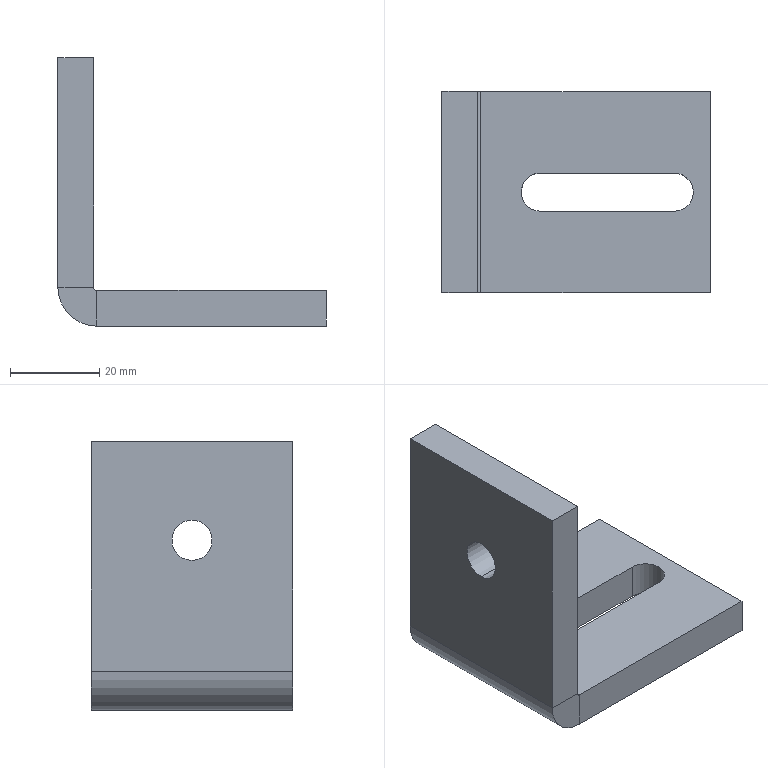Part | SolidWorks | features EdgeFlange 1, FlatPattern 1, HoleWzd 1, ICE 1, SMBaseFlange 1, SheetMetal 1 | 1 solid | 21 faces | box 60 x 45 x 60 mm | volume 36585 mm3 | plane 14 | cylinder 7 | commonest cylinder face diameters 8.5 x3 9 x2 1.473 x1 17.473 x1
STEP:
#1=CARTESIAN_POINT('',(64.788,13.156,0.));
#2=VERTEX_POINT('',#1);
#3=CARTESIAN_POINT('',(60.538,8.906,0.));
#4=VERTEX_POINT('',#3);
#5=CARTESIAN_POINT('',(64.788,8.906,0.));
#6=DIRECTION('',(0.,0.,1.));
#7=DIRECTION('',(1.,0.,0.));
#8=AXIS2_PLACEMENT_3D('',#5,#6,#7);
#9=CIRCLE('',#8,4.25);
#10=EDGE_CURVE('',#2,#4,#9,.T.);
#11=ORIENTED_EDGE('',*,*,#10,.T.);
#12=CARTESIAN_POINT('',(60.538,8.906,-8.));
#13=VERTEX_POINT('',#12);
#14=CARTESIAN_POINT('',(60.538,8.906,52.));
#15=DIRECTION('',(0.,0.,-1.));
#16=VECTOR('',#15,1000.);
#17=LINE('',#14,#16);
#18=EDGE_CURVE('',#4,#13,#17,.T.);
#19=ORIENTED_EDGE('',*,*,#18,.T.);
#20=CARTESIAN_POINT('',(64.788,13.156,-8.));
#21=VERTEX_POINT('',#20);
#22=CARTESIAN_POINT('',(64.788,8.906,-8.));
#23=DIRECTION('',(0.,0.,-1.));
#24=DIRECTION('',(-1.,0.,0.));
#25=AXIS2_PLACEMENT_3D('',#22,#23,#24);
#26=CIRCLE('',#25,4.25);
#27=EDGE_CURVE('',#13,#21,#26,.T.);
#28=ORIENTED_EDGE('',*,*,#27,.T.);
#29=CARTESIAN_POINT('',(64.788,13.156,52.));
#30=DIRECTION('',(0.,0.,-1.));
#31=VECTOR('',#30,1000.);
#32=LINE('',#29,#31);
#33=EDGE_CURVE('',#2,#21,#32,.T.);
#34=ORIENTED_EDGE('',*,*,#33,.F.);
#35=EDGE_LOOP('',(#11,#19,#28,#34));
#36=FACE_OUTER_BOUND('',#35,.T.);
#37=CARTESIAN_POINT('',(64.788,8.906,52.));
#38=DIRECTION('',(0.,0.,-1.));
#39=DIRECTION('',(-1.,0.,0.));
#40=AXIS2_PLACEMENT_3D('',#37,#38,#39);
#41=CYLINDRICAL_SURFACE('',#40,4.25);
#42=ADVANCED_FACE('',(#36),#41,.F.);
#43=CARTESIAN_POINT('',(42.788,8.906,34.5));
#44=VERTEX_POINT('',#43);
#45=CARTESIAN_POINT('',(42.788,8.906,25.5));
#46=VERTEX_POINT('',#45);
#47=CARTESIAN_POINT('',(42.788,8.906,30.));
#48=DIRECTION('',(1.,0.,0.));
#49=DIRECTION('',(0.,0.,-1.));
#50=AXIS2_PLACEMENT_3D('',#47,#48,#49);
#51=CIRCLE('',#50,4.5);
#52=EDGE_CURVE('',#44,#46,#51,.T.);
#53=ORIENTED_EDGE('',*,*,#52,.F.);
#54=CARTESIAN_POINT('',(50.788,8.906,34.5));
#55=VERTEX_POINT('',#54);
#56=CARTESIAN_POINT('',(50.788,8.906,34.5));
#57=DIRECTION('',(1.,0.,0.));
#58=VECTOR('',#57,1000.);
#59=LINE('',#56,#58);
#60=EDGE_CURVE('',#44,#55,#59,.T.);
#61=ORIENTED_EDGE('',*,*,#60,.T.);
#62=CARTESIAN_POINT('',(50.788,8.906,25.5));
#63=VERTEX_POINT('',#62);
#64=CARTESIAN_POINT('',(50.788,8.906,30.));
#65=DIRECTION('',(1.,0.,0.));
#66=DIRECTION('',(0.,0.,-1.));
#67=AXIS2_PLACEMENT_3D('',#64,#65,#66);
#68=CIRCLE('',#67,4.5);
#69=EDGE_CURVE('',#55,#63,#68,.T.);
#70=ORIENTED_EDGE('',*,*,#69,.T.);
#71=CARTESIAN_POINT('',(50.788,8.906,25.5));
#72=DIRECTION('',(1.,0.,0.));
#73=VECTOR('',#72,1000.);
#74=LINE('',#71,#73);
#75=EDGE_CURVE('',#46,#63,#74,.T.);
#76=ORIENTED_EDGE('',*,*,#75,.F.);
#77=EDGE_LOOP('',(#53,#61,#70,#76));
#78=FACE_OUTER_BOUND('',#77,.T.);
#79=CARTESIAN_POINT('',(50.788,8.906,30.));
#80=DIRECTION('',(1.,0.,0.));
#81=DIRECTION('',(0.,0.,-1.));
#82=AXIS2_PLACEMENT_3D('',#79,#80,#81);
#83=CYLINDRICAL_SURFACE('',#82,4.5);
#84=ADVANCED_FACE('',(#78),#83,.F.);
#85=CARTESIAN_POINT('',(51.525,-13.594,0.));
#86=VERTEX_POINT('',#85);
#87=CARTESIAN_POINT('',(102.788,-13.594,0.));
#88=VERTEX_POINT('',#87);
#89=CARTESIAN_POINT('',(42.788,-13.594,0.));
#90=DIRECTION('',(1.,0.,0.));
#91=VECTOR('',#90,1000.);
#92=LINE('',#89,#91);
#93=EDGE_CURVE('',#86,#88,#92,.T.);
#94=ORIENTED_EDGE('',*,*,#93,.F.);
#95=CARTESIAN_POINT('',(51.525,-13.594,-8.));
#96=VERTEX_POINT('',#95);
#97=CARTESIAN_POINT('',(51.525,-13.594,0.));
#98=DIRECTION('',(0.,0.,-1.));
#99=VECTOR('',#98,1000.);
#100=LINE('',#97,#99);
#101=EDGE_CURVE('',#86,#96,#100,.T.);
#102=ORIENTED_EDGE('',*,*,#101,.T.);
#103=CARTESIAN_POINT('',(102.788,-13.594,-8.));
#104=VERTEX_POINT('',#103);
#105=CARTESIAN_POINT('',(42.788,-13.594,-8.));
#106=DIRECTION('',(1.,0.,0.));
#107=VECTOR('',#106,1000.);
#108=LINE('',#105,#107);
#109=EDGE_CURVE('',#96,#104,#108,.T.);
#110=ORIENTED_EDGE('',*,*,#109,.T.);
#111=CARTESIAN_POINT('',(102.788,-13.594,-8.));
#112=DIRECTION('',(0.,0.,1.));
#113=VECTOR('',#112,1000.);
#114=LINE('',#111,#113);
#115=EDGE_CURVE('',#104,#88,#114,.T.);
#116=ORIENTED_EDGE('',*,*,#115,.T.);
#117=EDGE_LOOP('',(#94,#102,#110,#116));
#118=FACE_OUTER_BOUND('',#117,.T.);
#119=CARTESIAN_POINT('',(42.788,-13.594,-8.));
#120=DIRECTION('',(0.,-1.,0.));
#121=DIRECTION('',(0.,0.,-1.));
#122=AXIS2_PLACEMENT_3D('',#119,#120,#121);
#123=PLANE('',#122);
#124=ADVANCED_FACE('',(#118),#123,.T.);
#125=CARTESIAN_POINT('',(94.788,4.656,-8.));
#126=VERTEX_POINT('',#125);
#127=CARTESIAN_POINT('',(64.788,4.656,-8.));
#128=VERTEX_POINT('',#127);
#129=CARTESIAN_POINT('',(94.788,4.656,-8.));
#130=DIRECTION('',(-1.,0.,0.));
#131=VECTOR('',#130,1000.);
#132=LINE('',#129,#131);
#133=EDGE_CURVE('',#126,#128,#132,.T.);
#134=ORIENTED_EDGE('',*,*,#133,.F.);
#135=CARTESIAN_POINT('',(94.788,13.156,-8.));
#136=VERTEX_POINT('',#135);
#137=CARTESIAN_POINT('',(94.788,8.906,-8.));
#138=DIRECTION('',(0.,0.,-1.));
#139=DIRECTION('',(-1.,0.,0.));
#140=AXIS2_PLACEMENT_3D('',#137,#138,#139);
#141=CIRCLE('',#140,4.25);
#142=EDGE_CURVE('',#136,#126,#141,.T.);
#143=ORIENTED_EDGE('',*,*,#142,.F.);
#144=CARTESIAN_POINT('',(94.788,13.156,-8.));
#145=DIRECTION('',(1.,0.,0.));
#146=VECTOR('',#145,1000.);
#147=LINE('',#144,#146);
#148=EDGE_CURVE('',#21,#136,#147,.T.);
#149=ORIENTED_EDGE('',*,*,#148,.F.);
#150=ORIENTED_EDGE('',*,*,#27,.F.);
#151=CARTESIAN_POINT('',(64.788,8.906,-8.));
#152=DIRECTION('',(0.,0.,-1.));
#153=DIRECTION('',(-1.,0.,0.));
#154=AXIS2_PLACEMENT_3D('',#151,#152,#153);
#155=CIRCLE('',#154,4.25);
#156=EDGE_CURVE('',#128,#13,#155,.T.);
#157=ORIENTED_EDGE('',*,*,#156,.F.);
#158=EDGE_LOOP('',(#134,#143,#149,#150,#157));
#159=FACE_BOUND('',#158,.T.);
#160=CARTESIAN_POINT('',(51.525,31.406,-8.));
#161=VERTEX_POINT('',#160);
#162=CARTESIAN_POINT('',(51.525,-13.594,-8.));
#163=DIRECTION('',(0.,1.,0.));
#164=VECTOR('',#163,1000.);
#165=LINE('',#162,#164);
#166=EDGE_CURVE('',#96,#161,#165,.T.);
#167=ORIENTED_EDGE('',*,*,#166,.T.);
#168=CARTESIAN_POINT('',(102.788,31.406,-8.));
#169=VERTEX_POINT('',#168);
#170=CARTESIAN_POINT('',(42.788,31.406,-8.));
#171=DIRECTION('',(-1.,0.,0.));
#172=VECTOR('',#171,1000.);
#173=LINE('',#170,#172);
#174=EDGE_CURVE('',#169,#161,#173,.T.);
#175=ORIENTED_EDGE('',*,*,#174,.F.);
#176=CARTESIAN_POINT('',(102.788,31.406,-8.));
#177=DIRECTION('',(0.,1.,0.));
#178=VECTOR('',#177,1000.);
#179=LINE('',#176,#178);
#180=EDGE_CURVE('',#104,#169,#179,.T.);
#181=ORIENTED_EDGE('',*,*,#180,.F.);
#182=ORIENTED_EDGE('',*,*,#109,.F.);
#183=EDGE_LOOP('',(#167,#175,#181,#182));
#184=FACE_OUTER_BOUND('',#183,.T.);
#185=CARTESIAN_POINT('',(0.,0.,-8.));
#186=DIRECTION('',(0.,0.,1.));
#187=DIRECTION('',(1.,0.,0.));
#188=AXIS2_PLACEMENT_3D('',#185,#186,#187);
#189=PLANE('',#188);
#190=ADVANCED_FACE('',(#159,#184),#189,.F.);
#191=CARTESIAN_POINT('',(94.788,4.656,0.));
#192=VERTEX_POINT('',#191);
#193=CARTESIAN_POINT('',(94.788,13.156,0.));
#194=VERTEX_POINT('',#193);
#195=CARTESIAN_POINT('',(94.788,8.906,0.));
#196=DIRECTION('',(0.,0.,1.));
#197=DIRECTION('',(1.,0.,0.));
#198=AXIS2_PLACEMENT_3D('',#195,#196,#197);
#199=CIRCLE('',#198,4.25);
#200=EDGE_CURVE('',#192,#194,#199,.T.);
#201=ORIENTED_EDGE('',*,*,#200,.F.);
#202=CARTESIAN_POINT('',(64.788,4.656,0.));
#203=VERTEX_POINT('',#202);
#204=CARTESIAN_POINT('',(0.,4.656,0.));
#205=DIRECTION('',(1.,0.,0.));
#206=VECTOR('',#205,1000.);
#207=LINE('',#204,#206);
#208=EDGE_CURVE('',#203,#192,#207,.T.);
#209=ORIENTED_EDGE('',*,*,#208,.F.);
#210=CARTESIAN_POINT('',(64.788,8.906,0.));
#211=DIRECTION('',(0.,0.,1.));
#212=DIRECTION('',(1.,0.,0.));
#213=AXIS2_PLACEMENT_3D('',#210,#211,#212);
#214=CIRCLE('',#213,4.25);
#215=EDGE_CURVE('',#4,#203,#214,.T.);
#216=ORIENTED_EDGE('',*,*,#215,.F.);
#217=ORIENTED_EDGE('',*,*,#10,.F.);
#218=CARTESIAN_POINT('',(0.,13.156,0.));
#219=DIRECTION('',(-1.,0.,0.));
#220=VECTOR('',#219,1000.);
#221=LINE('',#218,#220);
#222=EDGE_CURVE('',#194,#2,#221,.T.);
#223=ORIENTED_EDGE('',*,*,#222,.F.);
#224=EDGE_LOOP('',(#201,#209,#216,#217,#223));
#225=FACE_BOUND('',#224,.T.);
#226=CARTESIAN_POINT('',(102.788,31.406,0.));
#227=VERTEX_POINT('',#226);
#228=CARTESIAN_POINT('',(51.525,31.406,0.));
#229=VERTEX_POINT('',#228);
#230=CARTESIAN_POINT('',(42.788,31.406,0.));
#231=DIRECTION('',(-1.,0.,0.));
#232=VECTOR('',#231,1000.);
#233=LINE('',#230,#232);
#234=EDGE_CURVE('',#227,#229,#233,.T.);
#235=ORIENTED_EDGE('',*,*,#234,.T.);
#236=CARTESIAN_POINT('',(51.525,-13.594,0.));
#237=DIRECTION('',(0.,1.,0.));
#238=VECTOR('',#237,1000.);
#239=LINE('',#236,#238);
#240=EDGE_CURVE('',#86,#229,#239,.T.);
#241=ORIENTED_EDGE('',*,*,#240,.F.);
#242=ORIENTED_EDGE('',*,*,#93,.T.);
#243=CARTESIAN_POINT('',(102.788,31.406,0.));
#244=DIRECTION('',(0.,1.,0.));
#245=VECTOR('',#244,1000.);
#246=LINE('',#243,#245);
#247=EDGE_CURVE('',#88,#227,#246,.T.);
#248=ORIENTED_EDGE('',*,*,#247,.T.);
#249=EDGE_LOOP('',(#235,#241,#242,#248));
#250=FACE_OUTER_BOUND('',#249,.T.);
#251=CARTESIAN_POINT('',(0.,0.,0.));
#252=DIRECTION('',(0.,0.,1.));
#253=DIRECTION('',(1.,0.,0.));
#254=AXIS2_PLACEMENT_3D('',#251,#252,#253);
#255=PLANE('',#254);
#256=ADVANCED_FACE('',(#225,#250),#255,.T.);
#257=ORIENTED_EDGE('',*,*,#247,.F.);
#258=ORIENTED_EDGE('',*,*,#115,.F.);
#259=ORIENTED_EDGE('',*,*,#180,.T.);
#260=CARTESIAN_POINT('',(102.788,31.406,-8.));
#261=DIRECTION('',(0.,0.,1.));
#262=VECTOR('',#261,1000.);
#263=LINE('',#260,#262);
#264=EDGE_CURVE('',#169,#227,#263,.T.);
#265=ORIENTED_EDGE('',*,*,#264,.T.);
#266=EDGE_LOOP('',(#257,#258,#259,#265));
#267=FACE_OUTER_BOUND('',#266,.T.);
#268=CARTESIAN_POINT('',(102.788,31.406,-8.));
#269=DIRECTION('',(1.,0.,0.));
#270=DIRECTION('',(0.,1.,0.));
#271=AXIS2_PLACEMENT_3D('',#268,#269,#270);
#272=PLANE('',#271);
#273=ADVANCED_FACE('',(#267),#272,.T.);
#274=CARTESIAN_POINT('',(51.525,31.406,0.));
#275=DIRECTION('',(0.,0.,-1.));
#276=VECTOR('',#275,1000.);
#277=LINE('',#274,#276);
#278=EDGE_CURVE('',#229,#161,#277,.T.);
#279=ORIENTED_EDGE('',*,*,#278,.F.);
#280=ORIENTED_EDGE('',*,*,#234,.F.);
#281=ORIENTED_EDGE('',*,*,#264,.F.);
#282=ORIENTED_EDGE('',*,*,#174,.T.);
#283=EDGE_LOOP('',(#279,#280,#281,#282));
#284=FACE_OUTER_BOUND('',#283,.T.);
#285=CARTESIAN_POINT('',(42.788,31.406,-8.));
#286=DIRECTION('',(0.,1.,0.));
#287=DIRECTION('',(0.,0.,1.));
#288=AXIS2_PLACEMENT_3D('',#285,#286,#287);
#289=PLANE('',#288);
#290=ADVANCED_FACE('',(#284),#289,.T.);
#291=CARTESIAN_POINT('',(50.788,31.406,0.7366));
#292=VERTEX_POINT('',#291);
#293=CARTESIAN_POINT('',(42.788,31.406,0.7366));
#294=VERTEX_POINT('',#293);
#295=CARTESIAN_POINT('',(42.788,31.406,0.7366));
#296=DIRECTION('',(-1.,0.,0.));
#297=VECTOR('',#296,1000.);
#298=LINE('',#295,#297);
#299=EDGE_CURVE('',#292,#294,#298,.T.);
#300=ORIENTED_EDGE('',*,*,#299,.F.);
#301=CARTESIAN_POINT('',(51.525,31.406,0.7366));
#302=DIRECTION('',(0.,1.,0.));
#303=DIRECTION('',(0.,0.,-1.));
#304=AXIS2_PLACEMENT_3D('',#301,#302,#303);
#305=CIRCLE('',#304,0.7366);
#306=EDGE_CURVE('',#229,#292,#305,.T.);
#307=ORIENTED_EDGE('',*,*,#306,.F.);
#308=ORIENTED_EDGE('',*,*,#278,.T.);
#309=CARTESIAN_POINT('',(51.525,31.406,0.7366));
#310=DIRECTION('',(0.,1.,0.));
#311=DIRECTION('',(0.,0.,-1.));
#312=AXIS2_PLACEMENT_3D('',#309,#310,#311);
#313=CIRCLE('',#312,8.737);
#314=EDGE_CURVE('',#161,#294,#313,.T.);
#315=ORIENTED_EDGE('',*,*,#314,.T.);
#316=EDGE_LOOP('',(#300,#307,#308,#315));
#317=FACE_OUTER_BOUND('',#316,.T.);
#318=CARTESIAN_POINT('',(51.525,31.406,0.7366));
#319=DIRECTION('',(0.,1.,0.));
#320=DIRECTION('',(0.,0.,1.));
#321=AXIS2_PLACEMENT_3D('',#318,#319,#320);
#322=PLANE('',#321);
#323=ADVANCED_FACE('',(#317),#322,.T.);
#324=CARTESIAN_POINT('',(50.788,-13.594,0.7366));
#325=VERTEX_POINT('',#324);
#326=CARTESIAN_POINT('',(51.525,-13.594,0.7366));
#327=DIRECTION('',(0.,-1.,0.));
#328=DIRECTION('',(0.,0.,-1.));
#329=AXIS2_PLACEMENT_3D('',#326,#327,#328);
#330=CIRCLE('',#329,0.7366);
#331=EDGE_CURVE('',#325,#86,#330,.T.);
#332=ORIENTED_EDGE('',*,*,#331,.F.);
#333=CARTESIAN_POINT('',(42.788,-13.594,0.7366));
#334=VERTEX_POINT('',#333);
#335=CARTESIAN_POINT('',(50.788,-13.594,0.7366));
#336=DIRECTION('',(-1.,0.,0.));
#337=VECTOR('',#336,1000.);
#338=LINE('',#335,#337);
#339=EDGE_CURVE('',#325,#334,#338,.T.);
#340=ORIENTED_EDGE('',*,*,#339,.T.);
#341=CARTESIAN_POINT('',(51.525,-13.594,0.7366));
#342=DIRECTION('',(0.,-1.,0.));
#343=DIRECTION('',(0.,0.,-1.));
#344=AXIS2_PLACEMENT_3D('',#341,#342,#343);
#345=CIRCLE('',#344,8.737);
#346=EDGE_CURVE('',#334,#96,#345,.T.);
#347=ORIENTED_EDGE('',*,*,#346,.T.);
#348=ORIENTED_EDGE('',*,*,#101,.F.);
#349=EDGE_LOOP('',(#332,#340,#347,#348));
#350=FACE_OUTER_BOUND('',#349,.T.);
#351=CARTESIAN_POINT('',(51.525,-13.594,0.7366));
#352=DIRECTION('',(0.,1.,0.));
#353=DIRECTION('',(0.,0.,1.));
#354=AXIS2_PLACEMENT_3D('',#351,#352,#353);
#355=PLANE('',#354);
#356=ADVANCED_FACE('',(#350),#355,.F.);
#357=ORIENTED_EDGE('',*,*,#166,.F.);
#358=ORIENTED_EDGE('',*,*,#346,.F.);
#359=CARTESIAN_POINT('',(42.788,31.406,0.7366));
#360=DIRECTION('',(0.,1.,0.));
#361=VECTOR('',#360,1000.);
#362=LINE('',#359,#361);
#363=EDGE_CURVE('',#334,#294,#362,.T.);
#364=ORIENTED_EDGE('',*,*,#363,.T.);
#365=ORIENTED_EDGE('',*,*,#314,.F.);
#366=EDGE_LOOP('',(#357,#358,#364,#365));
#367=FACE_OUTER_BOUND('',#366,.T.);
#368=CARTESIAN_POINT('',(51.525,-13.594,0.7366));
#369=DIRECTION('',(0.,-1.,0.));
#370=DIRECTION('',(-1.,0.,0.));
#371=AXIS2_PLACEMENT_3D('',#368,#369,#370);
#372=CYLINDRICAL_SURFACE('',#371,8.737);
#373=ADVANCED_FACE('',(#367),#372,.T.);
#374=ORIENTED_EDGE('',*,*,#240,.T.);
#375=ORIENTED_EDGE('',*,*,#306,.T.);
#376=CARTESIAN_POINT('',(50.788,31.406,0.7366));
#377=DIRECTION('',(0.,-1.,0.));
#378=VECTOR('',#377,1000.);
#379=LINE('',#376,#378);
#380=EDGE_CURVE('',#292,#325,#379,.T.);
#381=ORIENTED_EDGE('',*,*,#380,.T.);
#382=ORIENTED_EDGE('',*,*,#331,.T.);
#383=EDGE_LOOP('',(#374,#375,#381,#382));
#384=FACE_OUTER_BOUND('',#383,.T.);
#385=CARTESIAN_POINT('',(51.525,-13.594,0.7366));
#386=DIRECTION('',(0.,-1.,0.));
#387=DIRECTION('',(-1.,0.,0.));
#388=AXIS2_PLACEMENT_3D('',#385,#386,#387);
#389=CYLINDRICAL_SURFACE('',#388,0.7366);
#390=ADVANCED_FACE('',(#384),#389,.F.);
#391=ORIENTED_EDGE('',*,*,#299,.T.);
#392=CARTESIAN_POINT('',(42.788,31.406,52.));
#393=VERTEX_POINT('',#392);
#394=CARTESIAN_POINT('',(42.788,31.406,0.));
#395=DIRECTION('',(0.,0.,-1.));
#396=VECTOR('',#395,1000.);
#397=LINE('',#394,#396);
#398=EDGE_CURVE('',#393,#294,#397,.T.);
#399=ORIENTED_EDGE('',*,*,#398,.F.);
#400=CARTESIAN_POINT('',(50.788,31.406,52.));
#401=VERTEX_POINT('',#400);
#402=CARTESIAN_POINT('',(42.788,31.406,52.));
#403=DIRECTION('',(1.,0.,0.));
#404=VECTOR('',#403,1000.);
#405=LINE('',#402,#404);
#406=EDGE_CURVE('',#393,#401,#405,.T.);
#407=ORIENTED_EDGE('',*,*,#406,.T.);
#408=CARTESIAN_POINT('',(50.788,31.406,0.));
#409=DIRECTION('',(0.,0.,-1.));
#410=VECTOR('',#409,1000.);
#411=LINE('',#408,#410);
#412=EDGE_CURVE('',#401,#292,#411,.T.);
#413=ORIENTED_EDGE('',*,*,#412,.T.);
#414=EDGE_LOOP('',(#391,#399,#407,#413));
#415=FACE_OUTER_BOUND('',#414,.T.);
#416=CARTESIAN_POINT('',(42.788,31.406,0.));
#417=DIRECTION('',(0.,-1.,0.));
#418=DIRECTION('',(1.,0.,0.));
#419=AXIS2_PLACEMENT_3D('',#416,#417,#418);
#420=PLANE('',#419);
#421=ADVANCED_FACE('',(#415),#420,.F.);
#422=ORIENTED_EDGE('',*,*,#339,.F.);
#423=CARTESIAN_POINT('',(50.788,-13.594,52.));
#424=VERTEX_POINT('',#423);
#425=CARTESIAN_POINT('',(50.788,-13.594,52.));
#426=DIRECTION('',(0.,0.,1.));
#427=VECTOR('',#426,1000.);
#428=LINE('',#425,#427);
#429=EDGE_CURVE('',#325,#424,#428,.T.);
#430=ORIENTED_EDGE('',*,*,#429,.T.);
#431=CARTESIAN_POINT('',(42.788,-13.594,52.));
#432=VERTEX_POINT('',#431);
#433=CARTESIAN_POINT('',(42.788,-13.594,52.));
#434=DIRECTION('',(1.,0.,0.));
#435=VECTOR('',#434,1000.);
#436=LINE('',#433,#435);
#437=EDGE_CURVE('',#432,#424,#436,.T.);
#438=ORIENTED_EDGE('',*,*,#437,.F.);
#439=CARTESIAN_POINT('',(42.788,-13.594,0.));
#440=DIRECTION('',(0.,0.,1.));
#441=VECTOR('',#440,1000.);
#442=LINE('',#439,#441);
#443=EDGE_CURVE('',#334,#432,#442,.T.);
#444=ORIENTED_EDGE('',*,*,#443,.F.);
#445=EDGE_LOOP('',(#422,#430,#438,#444));
#446=FACE_OUTER_BOUND('',#445,.T.);
#447=CARTESIAN_POINT('',(42.788,-13.594,52.));
#448=DIRECTION('',(0.,1.,0.));
#449=DIRECTION('',(-1.,0.,0.));
#450=AXIS2_PLACEMENT_3D('',#447,#448,#449);
#451=PLANE('',#450);
#452=ADVANCED_FACE('',(#446),#451,.F.);
#453=CARTESIAN_POINT('',(42.788,8.906,30.));
#454=DIRECTION('',(1.,0.,0.));
#455=DIRECTION('',(0.,0.,-1.));
#456=AXIS2_PLACEMENT_3D('',#453,#454,#455);
#457=CIRCLE('',#456,4.5);
#458=EDGE_CURVE('',#46,#44,#457,.T.);
#459=ORIENTED_EDGE('',*,*,#458,.T.);
#460=ORIENTED_EDGE('',*,*,#52,.T.);
#461=EDGE_LOOP('',(#459,#460));
#462=FACE_BOUND('',#461,.T.);
#463=ORIENTED_EDGE('',*,*,#363,.F.);
#464=ORIENTED_EDGE('',*,*,#443,.T.);
#465=CARTESIAN_POINT('',(42.788,0.,52.));
#466=DIRECTION('',(0.,1.,0.));
#467=VECTOR('',#466,1000.);
#468=LINE('',#465,#467);
#469=EDGE_CURVE('',#432,#393,#468,.T.);
#470=ORIENTED_EDGE('',*,*,#469,.T.);
#471=ORIENTED_EDGE('',*,*,#398,.T.);
#472=EDGE_LOOP('',(#463,#464,#470,#471));
#473=FACE_OUTER_BOUND('',#472,.T.);
#474=CARTESIAN_POINT('',(42.788,0.,0.));
#475=DIRECTION('',(1.,0.,0.));
#476=DIRECTION('',(0.,0.,-1.));
#477=AXIS2_PLACEMENT_3D('',#474,#475,#476);
#478=PLANE('',#477);
#479=ADVANCED_FACE('',(#462,#473),#478,.F.);
#480=CARTESIAN_POINT('',(50.788,8.906,30.));
#481=DIRECTION('',(1.,0.,0.));
#482=DIRECTION('',(0.,0.,-1.));
#483=AXIS2_PLACEMENT_3D('',#480,#481,#482);
#484=CIRCLE('',#483,4.5);
#485=EDGE_CURVE('',#63,#55,#484,.T.);
#486=ORIENTED_EDGE('',*,*,#485,.F.);
#487=ORIENTED_EDGE('',*,*,#69,.F.);
#488=EDGE_LOOP('',(#486,#487));
#489=FACE_BOUND('',#488,.T.);
#490=ORIENTED_EDGE('',*,*,#429,.F.);
#491=ORIENTED_EDGE('',*,*,#380,.F.);
#492=ORIENTED_EDGE('',*,*,#412,.F.);
#493=CARTESIAN_POINT('',(50.788,31.406,52.));
#494=DIRECTION('',(0.,1.,0.));
#495=VECTOR('',#494,1000.);
#496=LINE('',#493,#495);
#497=EDGE_CURVE('',#424,#401,#496,.T.);
#498=ORIENTED_EDGE('',*,*,#497,.F.);
#499=EDGE_LOOP('',(#490,#491,#492,#498));
#500=FACE_OUTER_BOUND('',#499,.T.);
#501=CARTESIAN_POINT('',(50.788,0.,0.));
#502=DIRECTION('',(1.,0.,0.));
#503=DIRECTION('',(0.,0.,-1.));
#504=AXIS2_PLACEMENT_3D('',#501,#502,#503);
#505=PLANE('',#504);
#506=ADVANCED_FACE('',(#489,#500),#505,.T.);
#507=ORIENTED_EDGE('',*,*,#497,.T.);
#508=ORIENTED_EDGE('',*,*,#406,.F.);
#509=ORIENTED_EDGE('',*,*,#469,.F.);
#510=ORIENTED_EDGE('',*,*,#437,.T.);
#511=EDGE_LOOP('',(#507,#508,#509,#510));
#512=FACE_OUTER_BOUND('',#511,.T.);
#513=CARTESIAN_POINT('',(42.788,31.406,52.));
#514=DIRECTION('',(0.,0.,-1.));
#515=DIRECTION('',(-1.,0.,0.));
#516=AXIS2_PLACEMENT_3D('',#513,#514,#515);
#517=PLANE('',#516);
#518=ADVANCED_FACE('',(#512),#517,.F.);
#519=ORIENTED_EDGE('',*,*,#60,.F.);
#520=ORIENTED_EDGE('',*,*,#458,.F.);
#521=ORIENTED_EDGE('',*,*,#75,.T.);
#522=ORIENTED_EDGE('',*,*,#485,.T.);
#523=EDGE_LOOP('',(#519,#520,#521,#522));
#524=FACE_OUTER_BOUND('',#523,.T.);
#525=CARTESIAN_POINT('',(50.788,8.906,30.));
#526=DIRECTION('',(1.,0.,0.));
#527=DIRECTION('',(0.,0.,-1.));
#528=AXIS2_PLACEMENT_3D('',#525,#526,#527);
#529=CYLINDRICAL_SURFACE('',#528,4.5);
#530=ADVANCED_FACE('',(#524),#529,.F.);
#531=ORIENTED_EDGE('',*,*,#200,.T.);
#532=CARTESIAN_POINT('',(94.788,13.156,52.));
#533=DIRECTION('',(0.,0.,-1.));
#534=VECTOR('',#533,1000.);
#535=LINE('',#532,#534);
#536=EDGE_CURVE('',#194,#136,#535,.T.);
#537=ORIENTED_EDGE('',*,*,#536,.T.);
#538=ORIENTED_EDGE('',*,*,#142,.T.);
#539=CARTESIAN_POINT('',(94.788,4.656,52.));
#540=DIRECTION('',(0.,0.,-1.));
#541=VECTOR('',#540,1000.);
#542=LINE('',#539,#541);
#543=EDGE_CURVE('',#192,#126,#542,.T.);
#544=ORIENTED_EDGE('',*,*,#543,.F.);
#545=EDGE_LOOP('',(#531,#537,#538,#544));
#546=FACE_OUTER_BOUND('',#545,.T.);
#547=CARTESIAN_POINT('',(94.788,8.906,52.));
#548=DIRECTION('',(0.,0.,-1.));
#549=DIRECTION('',(-1.,0.,0.));
#550=AXIS2_PLACEMENT_3D('',#547,#548,#549);
#551=CYLINDRICAL_SURFACE('',#550,4.25);
#552=ADVANCED_FACE('',(#546),#551,.F.);
#553=ORIENTED_EDGE('',*,*,#222,.T.);
#554=ORIENTED_EDGE('',*,*,#33,.T.);
#555=ORIENTED_EDGE('',*,*,#148,.T.);
#556=ORIENTED_EDGE('',*,*,#536,.F.);
#557=EDGE_LOOP('',(#553,#554,#555,#556));
#558=FACE_OUTER_BOUND('',#557,.T.);
#559=CARTESIAN_POINT('',(94.788,13.156,52.));
#560=DIRECTION('',(0.,1.,0.));
#561=DIRECTION('',(0.,0.,1.));
#562=AXIS2_PLACEMENT_3D('',#559,#560,#561);
#563=PLANE('',#562);
#564=ADVANCED_FACE('',(#558),#563,.F.);
#565=ORIENTED_EDGE('',*,*,#18,.F.);
#566=ORIENTED_EDGE('',*,*,#215,.T.);
#567=CARTESIAN_POINT('',(64.788,4.656,52.));
#568=DIRECTION('',(0.,0.,-1.));
#569=VECTOR('',#568,1000.);
#570=LINE('',#567,#569);
#571=EDGE_CURVE('',#203,#128,#570,.T.);
#572=ORIENTED_EDGE('',*,*,#571,.T.);
#573=ORIENTED_EDGE('',*,*,#156,.T.);
#574=EDGE_LOOP('',(#565,#566,#572,#573));
#575=FACE_OUTER_BOUND('',#574,.T.);
#576=CARTESIAN_POINT('',(64.788,8.906,52.));
#577=DIRECTION('',(0.,0.,-1.));
#578=DIRECTION('',(-1.,0.,0.));
#579=AXIS2_PLACEMENT_3D('',#576,#577,#578);
#580=CYLINDRICAL_SURFACE('',#579,4.25);
#581=ADVANCED_FACE('',(#575),#580,.F.);
#582=ORIENTED_EDGE('',*,*,#208,.T.);
#583=ORIENTED_EDGE('',*,*,#543,.T.);
#584=ORIENTED_EDGE('',*,*,#133,.T.);
#585=ORIENTED_EDGE('',*,*,#571,.F.);
#586=EDGE_LOOP('',(#582,#583,#584,#585));
#587=FACE_OUTER_BOUND('',#586,.T.);
#588=CARTESIAN_POINT('',(94.788,4.656,52.));
#589=DIRECTION('',(0.,-1.,0.));
#590=DIRECTION('',(0.,0.,-1.));
#591=AXIS2_PLACEMENT_3D('',#588,#589,#590);
#592=PLANE('',#591);
#593=ADVANCED_FACE('',(#587),#592,.F.);
#594=CLOSED_SHELL('',(#42,#84,#124,#190,#256,#273,#290,#323,#356,#373,#390,#421,#452,#479,#506,#518,#530,#552,#564,#581,#593));
#595=MANIFOLD_SOLID_BREP('',#594);
#596=CARTESIAN_POINT('',(0.,0.,0.));
#597=DIRECTION('',(0.,0.,1.));
#598=DIRECTION('',(1.,0.,0.));
#599=AXIS2_PLACEMENT_3D('',#596,#597,#598);
#600=(LENGTH_UNIT()NAMED_UNIT(*)SI_UNIT(.MILLI.,.METRE.));
#601=UNCERTAINTY_MEASURE_WITH_UNIT(LENGTH_MEASURE(0.00001),#600,'','');
#602=(NAMED_UNIT(*)PLANE_ANGLE_UNIT()SI_UNIT($,.RADIAN.));
#603=(NAMED_UNIT(*)SI_UNIT($,.STERADIAN.)SOLID_ANGLE_UNIT());
#604=(GEOMETRIC_REPRESENTATION_CONTEXT(3)GLOBAL_UNCERTAINTY_ASSIGNED_CONTEXT((#601))GLOBAL_UNIT_ASSIGNED_CONTEXT((#600,#602,#603))REPRESENTATION_CONTEXT('',''));
#605=ADVANCED_BREP_SHAPE_REPRESENTATION('',(#595,#599),#604);